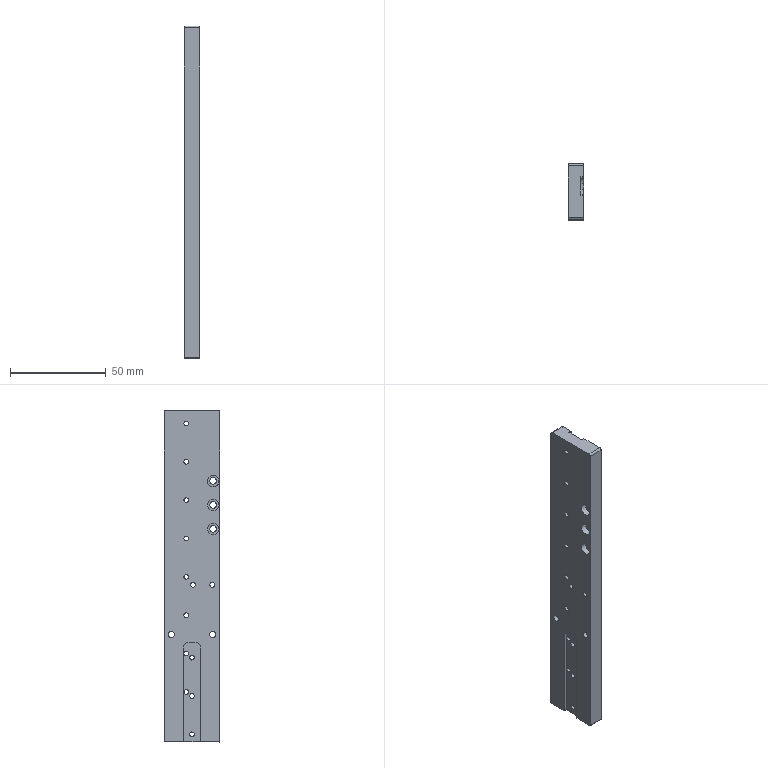CAM job | NX | 3+2 milling, drilling | part box 8 x 29 x 173.1 mm | stock box 10 x 30 x 178.1 mm
Tools:
number,name,description,diameter,corner_radius,flute_length,length,flutes
4,D4,平底铣刀-粗,4.0,0.0,25.0,75.0,2
6,D6,平底铣刀-粗,6.0,0.0,25.0,75.0,2
9,D10,平底铣刀-粗,10.0,0.0,35.0,75.0,2
7,D6-J,平底铣刀-精,6.0,0.0,25.0,75.0,2
10,D10-J,平底铣刀-精,10.0,0.0,35.0,75.0,2
1,D80R0.8飞刀,圆鼻刀-粗,80.0,0.8,50.0,75.0,2
1,D80R0.8飞刀-J,圆鼻刀-精,80.0,0.8,50.0,75.0,2
2,D6倒角刀,倒角刀,6.0,0.0,3.0,25.0,2
20,M3X0.5,丝锥,2.5,0.0,35.0,50.0,2
21,M4X0.7,丝锥,3.3,0.0,35.0,50.0,2
12,ZT2.5,钻头,2.5,0.0,35.0,50.0,2
17,ZT3.5,钻头,3.5,0.0,35.0,50.0,2
13,钻头3.3,Twist Drill 3.3 mm,3.3,0.0,35.0,35.008,2
Operations:
program,operation,operation_type,tool,method,geometry_group,spindle_rpm,surface_speed,feed_per_tooth,feed_cut,feed_plunge,cut_length_mm,path_length_mm,cut_time_min,machine_time_min
B,底壁铣飞面一刀开粗_COPY,VolumeBased25DMillingOperation,D80R0.8飞刀,分层开粗-切深K-步距G,W-B,2800.0,703.696,0.5357,3000.0,100.0,1125.176,1991.434,0.3751,0.4617
B,底壁铣飞面一刀精光_COPY,VolumeBased25DMillingOperation,D80R0.8飞刀-J,侧刃精光-切深K-步距G,W-B,4000.0,1005.28,0.125,1000.0,100.0,281.098,317.098,0.2811,0.2847
B,底壁粗_1_COPY,VolumeBased25DMillingOperation,D6,METHOD,W-B,6000.0,113.0,0.2083,1200.0,100.0,1303.966,1488.991,1.087,1.105
B,钻倒角_3,Operation,D6倒角刀,METHOD,W-B,8000.0,150.796,0.0625,1000.0,0.0,47.5,349.87,0.0475,0.0777
B,钻倒角_4,Operation,D6倒角刀,METHOD,W-B,8000.0,150.796,0.0625,1000.0,0.0,10.4,85.508,0.0104,0.0179
B,钻倒角_5,Operation,D6倒角刀,METHOD,W-B,8000.0,150.796,0.0625,1000.0,0.0,15.15,102.01,0.0151,0.0238
B,平面去毛刺6X45L_COPY,SurfaceContour,D6倒角刀,爬面_倒角-切深0-步距G,W-B,6500.0,122.519,0.1154,1500.0,100.0,783.284,1119.734,0.5222,0.5558
B,底侧精_3_COPY,VolumeBased25DMillingOperation,D6-J,METHOD,W-B,6000.0,113.0,0.2083,1200.0,100.0,331.249,373.249,0.276,0.2802
A,顶面开粗,FaceMilling,D80R0.8飞刀,分层开粗-切深K-步距G,W-A,4000.0,1005.31,0.375,3000.0,100.0,267.1,302.9,0.089,0.0926
A,顶面,FaceMilling,D80R0.8飞刀,侧刃精光-切深K-步距G,W-A,4000.0,1005.31,0.125,1000.0,100.0,267.1,303.1,0.2671,0.2707
A,外形粗_2,VolumeBased25DMillingOperation,D10,METHOD,W-A,8000.0,251.327,0.3125,5000.0,80.0,5223.326,5269.926,1.045,1.049
A,打点-深0.8,Operation,D6倒角刀,NONE,W-A,8000.0,150.796,0.0312,500.0,90.0,32.4,368.018,0.0648,0.0984
A,通孔-M3螺纹底孔,Operation,ZT2.5,NONE,W-A,3000.0,23.562,0.05,300.0,90.0,195.0,624.398,0.65,0.6929
A,通孔-M4螺纹底孔,Operation,钻头3.3,NONE,W-A,3000.0,31.102,0.05,300.0,90.0,29.983,122.489,0.0999,0.1092
A,沉头孔-钻孔0段,Operation,ZT3.5,NONE,W-A,2800.0,30.788,0.0179,100.0,90.0,36.154,139.389,0.3615,0.3719
A,钻倒角_1,Operation,D6倒角刀,METHOD,W-A,8000.0,150.796,0.0312,500.0,0.0,61.75,386.447,0.1235,0.156
A,钻倒角_2,Operation,D6倒角刀,METHOD,W-A,8000.0,150.796,0.0312,500.0,0.0,10.4,85.508,0.0208,0.0283
A,通孔-攻牙M3,Operation,M3X0.5,METHOD,W-A,800.0,6.283,0.0003,0.5,90.0,141.0,516.398,282.0,282.038
A,通孔-攻牙M4,Operation,M4X0.7,METHOD,W-A,600.0,6.22,0.0006,0.7,90.0,24.0,110.523,34.286,34.294
A,底壁粗_1,VolumeBased25DMillingOperation,D6,METHOD,W-A,6000.0,113.0,0.2083,1200.0,100.0,447.901,632.926,0.3733,0.3918
A,铣孔开粗D4_1,CylinderMilling,D4,NONE,W-A,8000.0,100.531,0.075,1200.0,100.0,223.646,376.146,0.1864,0.2016
A,铣孔精光D4_1,CylinderMilling,D4,精光步距切深关,W-A,8000.0,100.531,0.0312,500.0,100.0,44.823,197.323,0.0896,0.1049
A,铣倒角_1,PlanarMilling,D6倒角刀,NONE,W-A,8000.0,150.796,0.0312,500.0,100.0,83.054,223.023,0.1661,0.1801
A,仅选体,SurfaceContour,D6倒角刀,METHOD,W-A,8000.0,150.796,0.1875,3000.0,100.0,535.071,695.787,0.1784,0.1944
A,底侧精_3,VolumeBased25DMillingOperation,D6-J,METHOD,W-A,6000.0,113.0,0.2083,1200.0,100.0,117.232,159.232,0.0977,0.1019
A,外形半精_2,VolumeBased25DMillingOperation,D10-J,METHOD,W-A,8000.0,251.327,0.0625,1000.0,100.0,439.481,494.681,0.4395,0.445